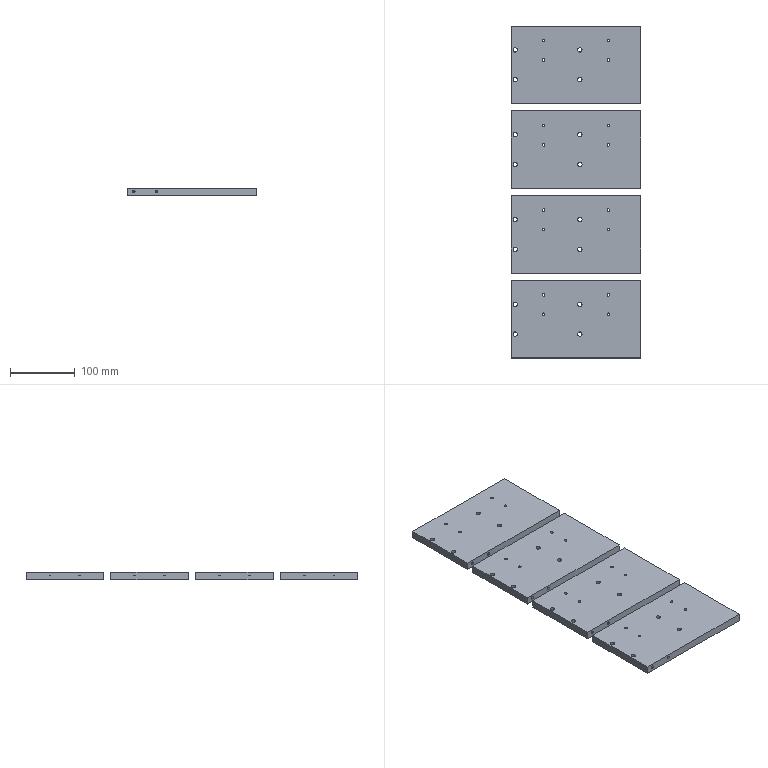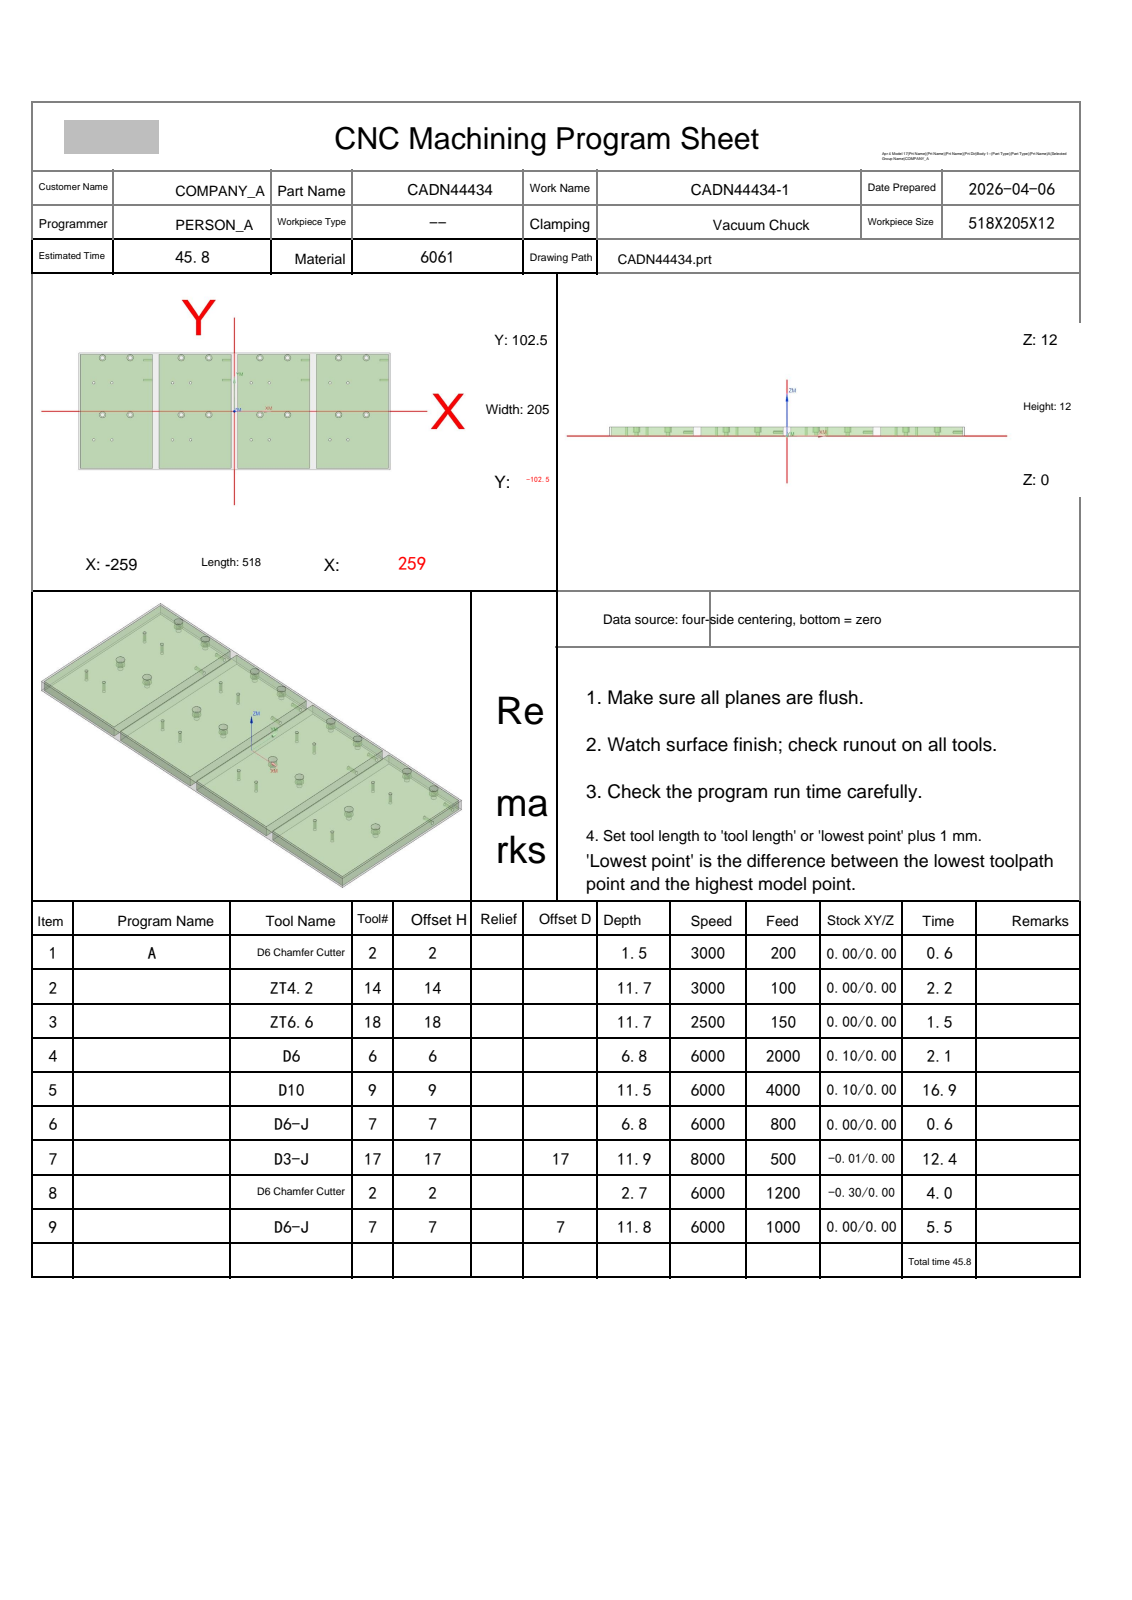NC program | NX | posted by the shop | part box 200 x 513 x 12 mm
Lines 1 to 1643 of 7719, first 1345 of 1641 lines:
%
O0001
(Machine time: 47.09 MIN)
(===Total Tool:7===)
(T2=D6 Chamfer Cutter D=6. R=0. D- H02 Z=9.33  )
(T14=ZT4.2  D=4.2  DR_a=118 D-  H14 Z=0.3   )
(T18=ZT6.6  D=6.6  DR_a=118 D-  H18 Z=0.3   )
(T6=D6      D=6.   R=0.   D-  H06 Z=5.2   )
(T9=D10     D=10.  R=0.   D-  H09 Z=0.5   )
(T7=D6-J    D=6.   R=0.   D-  H07 Z=0.2   )
(T17=D3-J   D=3.   R=0.   D17 H17 Z=0.15  )
G80 G90 G17 G49 G40
G91 G28 Z0
M01
N1 T02 M06
(D6 Chamfer Cutter  D=6. R=0. H=02 ce=0.00 di=0.00)
G00 G90 G54 X-204. Y-50. M03 S3000
G43 H02 Z32.
M08
G98 G81 X-204. Y-50. Z10.5 R13. F200.
X-234.
X-219.5 Y-6.
X-173.5
X-204. Y50.
X-234.
X-219.5 Y94.
X-173.5
X-88.5
X-42.5
X-73. Y50.
X-103.
X-88.5 Y-6.
X-103. Y-50.
X-73.
X-42.5 Y-6.
X28. Y-50.
X58.
X42.5 Y-6.
X88.5
X58. Y50.
X28.
X42.5 Y94.
X88.5
X173.5
X219.5
X189. Y50.
X159.
X173.5 Y-6.
X219.5
X189. Y-50.
X159.
G80
G00 Z32.
G91 G28 Z0.0
M05
M09
G91 G28 Z0.0
M01
N2 T14 M06
(ZT4.2 D=4.2 DR_a=118 H=14)
G00 G90 G54 X-73. Y-50. M03 S3000
G43 H14 Z32.
M08
G98 G83 X-73. Y-50. Z.3 R13. F100. Q1.5
X-103.
X-204.
X-234.
Y50.
X-204.
X-103.
X-73.
X28.
X58.
X159.
X189.
Y-50.
X159.
X58.
X28.
G80
G00 Z32.
G91 G28 Z0.0
M05
M09
G91 G28 Z0.0
M01
N3 T18 M06
(ZT6.6 D=6.6 DR_a=118 H=18)
G00 G90 G54 X219.5 Y94. M03 S2500
G43 H18 Z32.
M08
G98 G83 X219.5 Y94. Z.3 R13. F150. Q3.
X173.5
X88.5
X42.5
X-42.5
X-88.5
X-173.5
X-219.5
Y-6.
X-173.5
X-88.5
X-42.5
X42.5
X88.5
X173.5
X219.5
G80
G00 Z32.
G91 G28 Z0.0
M05
M09
G91 G28 Z0.0
M01
N4 T06 M06
(D6  D=6. R=0. H=06 ce=0.10 di=0.00)
G00 G90 G54 X88.5 Y-6. M03 S6000
G43 H06 Z32.
M08
Z12.3
G03 X87.3 Y-7.2 I0.0 J-1.2 F2000.
X88.5 Y-8.4 I1.2 J0.0
X88.5 Y-8.4 Z11.8 I0.0 J2.4
X88.5 Y-8.4 Z11.3 I0.0 J2.4
X88.5 Y-8.4 Z10.8 I0.0 J2.4
X88.5 Y-8.4 Z10.3 I0.0 J2.4
X88.5 Y-8.4 Z9.8 I0.0 J2.4
X88.5 Y-8.4 Z9.3 I0.0 J2.4
X88.5 Y-8.4 Z8.8 I0.0 J2.4
X88.5 Y-8.4 Z8.3 I0.0 J2.4
X88.5 Y-8.4 Z7.8 I0.0 J2.4
X88.5 Y-8.4 Z7.3 I0.0 J2.4
X88.5 Y-8.4 Z6.8 I0.0 J2.4
X88.5 Y-8.4 Z6.3 I0.0 J2.4
X88.5 Y-8.4 Z5.8 I0.0 J2.4
X88.5 Y-8.4 Z5.3 I0.0 J2.4
X90.783 Y-6.742 Z5.2 I0.0 J2.4
X90.9 Y-6. I-2.283 J.742
X88.5 Y-3.6 I-2.4 J0.0
X86.1 Y-6. I0.0 J-2.4
X88.5 Y-8.4 I2.4 J0.0
X90.783 Y-6.742 I0.0 J2.4
X90.841 Y-6.371 I-1.141 J.371
X89.641 Y-5.171 I-1.2 J0.0
X88.5 Y-6. I0.0 J-1.2
G00 Z32.
X42.5
Z12.3
G03 X41.3 Y-7.2 I0.0 J-1.2
X42.5 Y-8.4 I1.2 J0.0
X42.5 Y-8.4 Z11.8 I0.0 J2.4
X42.5 Y-8.4 Z11.3 I0.0 J2.4
X42.5 Y-8.4 Z10.8 I0.0 J2.4
X42.5 Y-8.4 Z10.3 I0.0 J2.4
X42.5 Y-8.4 Z9.8 I0.0 J2.4
X42.5 Y-8.4 Z9.3 I0.0 J2.4
X42.5 Y-8.4 Z8.8 I0.0 J2.4
X42.5 Y-8.4 Z8.3 I0.0 J2.4
X42.5 Y-8.4 Z7.8 I0.0 J2.4
X42.5 Y-8.4 Z7.3 I0.0 J2.4
X42.5 Y-8.4 Z6.8 I0.0 J2.4
X42.5 Y-8.4 Z6.3 I0.0 J2.4
X42.5 Y-8.4 Z5.8 I0.0 J2.4
X42.5 Y-8.4 Z5.3 I0.0 J2.4
X44.783 Y-6.742 Z5.2 I0.0 J2.4
X44.9 Y-6. I-2.283 J.742
X42.5 Y-3.6 I-2.4 J0.0
X40.1 Y-6. I0.0 J-2.4
X42.5 Y-8.4 I2.4 J0.0
X44.783 Y-6.742 I0.0 J2.4
X44.841 Y-6.371 I-1.141 J.371
X43.641 Y-5.171 I-1.2 J0.0
X42.5 Y-6. I0.0 J-1.2
G00 Z32.
X-42.5
Z12.3
G03 X-43.7 Y-7.2 I0.0 J-1.2
X-42.5 Y-8.4 I1.2 J0.0
X-42.5 Y-8.4 Z11.8 I0.0 J2.4
X-42.5 Y-8.4 Z11.3 I0.0 J2.4
X-42.5 Y-8.4 Z10.8 I0.0 J2.4
X-42.5 Y-8.4 Z10.3 I0.0 J2.4
X-42.5 Y-8.4 Z9.8 I0.0 J2.4
X-42.5 Y-8.4 Z9.3 I0.0 J2.4
X-42.5 Y-8.4 Z8.8 I0.0 J2.4
X-42.5 Y-8.4 Z8.3 I0.0 J2.4
X-42.5 Y-8.4 Z7.8 I0.0 J2.4
X-42.5 Y-8.4 Z7.3 I0.0 J2.4
X-42.5 Y-8.4 Z6.8 I0.0 J2.4
X-42.5 Y-8.4 Z6.3 I0.0 J2.4
X-42.5 Y-8.4 Z5.8 I0.0 J2.4
X-42.5 Y-8.4 Z5.3 I0.0 J2.4
X-40.217 Y-6.742 Z5.2 I0.0 J2.4
X-40.1 Y-6. I-2.283 J.742
X-42.5 Y-3.6 I-2.4 J0.0
X-44.9 Y-6. I0.0 J-2.4
X-42.5 Y-8.4 I2.4 J0.0
X-40.217 Y-6.742 I0.0 J2.4
X-40.159 Y-6.371 I-1.141 J.371
X-41.359 Y-5.171 I-1.2 J0.0
X-42.5 Y-6. I0.0 J-1.2
G00 Z32.
X-88.5
Z12.3
G03 X-89.7 Y-7.2 I0.0 J-1.2
X-88.5 Y-8.4 I1.2 J0.0
X-88.5 Y-8.4 Z11.8 I0.0 J2.4
X-88.5 Y-8.4 Z11.3 I0.0 J2.4
X-88.5 Y-8.4 Z10.8 I0.0 J2.4
X-88.5 Y-8.4 Z10.3 I0.0 J2.4
X-88.5 Y-8.4 Z9.8 I0.0 J2.4
X-88.5 Y-8.4 Z9.3 I0.0 J2.4
X-88.5 Y-8.4 Z8.8 I0.0 J2.4
X-88.5 Y-8.4 Z8.3 I0.0 J2.4
X-88.5 Y-8.4 Z7.8 I0.0 J2.4
X-88.5 Y-8.4 Z7.3 I0.0 J2.4
X-88.5 Y-8.4 Z6.8 I0.0 J2.4
X-88.5 Y-8.4 Z6.3 I0.0 J2.4
X-88.5 Y-8.4 Z5.8 I0.0 J2.4
X-88.5 Y-8.4 Z5.3 I0.0 J2.4
X-86.217 Y-6.742 Z5.2 I0.0 J2.4
X-86.1 Y-6. I-2.283 J.742
X-88.5 Y-3.6 I-2.4 J0.0
X-90.9 Y-6. I0.0 J-2.4
X-88.5 Y-8.4 I2.4 J0.0
X-86.217 Y-6.742 I0.0 J2.4
X-86.159 Y-6.371 I-1.141 J.371
X-87.359 Y-5.171 I-1.2 J0.0
X-88.5 Y-6. I0.0 J-1.2
G00 Z32.
X-173.5
Z12.3
G03 X-174.7 Y-7.2 I0.0 J-1.2
X-173.5 Y-8.4 I1.2 J0.0
X-173.5 Y-8.4 Z11.8 I0.0 J2.4
X-173.5 Y-8.4 Z11.3 I0.0 J2.4
X-173.5 Y-8.4 Z10.8 I0.0 J2.4
X-173.5 Y-8.4 Z10.3 I0.0 J2.4
X-173.5 Y-8.4 Z9.8 I0.0 J2.4
X-173.5 Y-8.4 Z9.3 I0.0 J2.4
X-173.5 Y-8.4 Z8.8 I0.0 J2.4
X-173.5 Y-8.4 Z8.3 I0.0 J2.4
X-173.5 Y-8.4 Z7.8 I0.0 J2.4
X-173.5 Y-8.4 Z7.3 I0.0 J2.4
X-173.5 Y-8.4 Z6.8 I0.0 J2.4
X-173.5 Y-8.4 Z6.3 I0.0 J2.4
X-173.5 Y-8.4 Z5.8 I0.0 J2.4
X-173.5 Y-8.4 Z5.3 I0.0 J2.4
X-171.217 Y-6.742 Z5.2 I0.0 J2.4
X-171.1 Y-6. I-2.283 J.742
X-173.5 Y-3.6 I-2.4 J0.0
X-175.9 Y-6. I0.0 J-2.4
X-173.5 Y-8.4 I2.4 J0.0
X-171.217 Y-6.742 I0.0 J2.4
X-171.159 Y-6.371 I-1.141 J.371
X-172.359 Y-5.171 I-1.2 J0.0
X-173.5 Y-6. I0.0 J-1.2
G00 Z32.
X-219.5
Z12.3
G03 X-220.7 Y-7.2 I0.0 J-1.2
X-219.5 Y-8.4 I1.2 J0.0
X-219.5 Y-8.4 Z11.8 I0.0 J2.4
X-219.5 Y-8.4 Z11.3 I0.0 J2.4
X-219.5 Y-8.4 Z10.8 I0.0 J2.4
X-219.5 Y-8.4 Z10.3 I0.0 J2.4
X-219.5 Y-8.4 Z9.8 I0.0 J2.4
X-219.5 Y-8.4 Z9.3 I0.0 J2.4
X-219.5 Y-8.4 Z8.8 I0.0 J2.4
X-219.5 Y-8.4 Z8.3 I0.0 J2.4
X-219.5 Y-8.4 Z7.8 I0.0 J2.4
X-219.5 Y-8.4 Z7.3 I0.0 J2.4
X-219.5 Y-8.4 Z6.8 I0.0 J2.4
X-219.5 Y-8.4 Z6.3 I0.0 J2.4
X-219.5 Y-8.4 Z5.8 I0.0 J2.4
X-219.5 Y-8.4 Z5.3 I0.0 J2.4
X-217.217 Y-6.742 Z5.2 I0.0 J2.4
X-217.1 Y-6. I-2.283 J.742
X-219.5 Y-3.6 I-2.4 J0.0
X-221.9 Y-6. I0.0 J-2.4
X-219.5 Y-8.4 I2.4 J0.0
X-217.217 Y-6.742 I0.0 J2.4
X-217.159 Y-6.371 I-1.141 J.371
X-218.359 Y-5.171 I-1.2 J0.0
X-219.5 Y-6. I0.0 J-1.2
G00 Z32.
Y94.
Z12.3
G03 X-220.7 Y92.8 I0.0 J-1.2
X-219.5 Y91.6 I1.2 J0.0
X-219.5 Y91.6 Z11.8 I0.0 J2.4
X-219.5 Y91.6 Z11.3 I0.0 J2.4
X-219.5 Y91.6 Z10.8 I0.0 J2.4
X-219.5 Y91.6 Z10.3 I0.0 J2.4
X-219.5 Y91.6 Z9.8 I0.0 J2.4
X-219.5 Y91.6 Z9.3 I0.0 J2.4
X-219.5 Y91.6 Z8.8 I0.0 J2.4
X-219.5 Y91.6 Z8.3 I0.0 J2.4
X-219.5 Y91.6 Z7.8 I0.0 J2.4
X-219.5 Y91.6 Z7.3 I0.0 J2.4
X-219.5 Y91.6 Z6.8 I0.0 J2.4
X-219.5 Y91.6 Z6.3 I0.0 J2.4
X-219.5 Y91.6 Z5.8 I0.0 J2.4
X-219.5 Y91.6 Z5.3 I0.0 J2.4
X-217.217 Y93.258 Z5.2 I0.0 J2.4
X-217.1 Y94. I-2.283 J.742
X-219.5 Y96.4 I-2.4 J0.0
X-221.9 Y94. I0.0 J-2.4
X-219.5 Y91.6 I2.4 J0.0
X-217.217 Y93.258 I0.0 J2.4
X-217.159 Y93.629 I-1.141 J.371
X-218.359 Y94.829 I-1.2 J0.0
X-219.5 Y94. I0.0 J-1.2
G00 Z32.
X-173.5
Z12.3
G03 X-174.7 Y92.8 I0.0 J-1.2
X-173.5 Y91.6 I1.2 J0.0
X-173.5 Y91.6 Z11.8 I0.0 J2.4
X-173.5 Y91.6 Z11.3 I0.0 J2.4
X-173.5 Y91.6 Z10.8 I0.0 J2.4
X-173.5 Y91.6 Z10.3 I0.0 J2.4
X-173.5 Y91.6 Z9.8 I0.0 J2.4
X-173.5 Y91.6 Z9.3 I0.0 J2.4
X-173.5 Y91.6 Z8.8 I0.0 J2.4
X-173.5 Y91.6 Z8.3 I0.0 J2.4
X-173.5 Y91.6 Z7.8 I0.0 J2.4
X-173.5 Y91.6 Z7.3 I0.0 J2.4
X-173.5 Y91.6 Z6.8 I0.0 J2.4
X-173.5 Y91.6 Z6.3 I0.0 J2.4
X-173.5 Y91.6 Z5.8 I0.0 J2.4
X-173.5 Y91.6 Z5.3 I0.0 J2.4
X-171.217 Y93.258 Z5.2 I0.0 J2.4
X-171.1 Y94. I-2.283 J.742
X-173.5 Y96.4 I-2.4 J0.0
X-175.9 Y94. I0.0 J-2.4
X-173.5 Y91.6 I2.4 J0.0
X-171.217 Y93.258 I0.0 J2.4
X-171.159 Y93.629 I-1.141 J.371
X-172.359 Y94.829 I-1.2 J0.0
X-173.5 Y94. I0.0 J-1.2
G00 Z32.
X-88.5
Z12.3
G03 X-89.7 Y92.8 I0.0 J-1.2
X-88.5 Y91.6 I1.2 J0.0
X-88.5 Y91.6 Z11.8 I0.0 J2.4
X-88.5 Y91.6 Z11.3 I0.0 J2.4
X-88.5 Y91.6 Z10.8 I0.0 J2.4
X-88.5 Y91.6 Z10.3 I0.0 J2.4
X-88.5 Y91.6 Z9.8 I0.0 J2.4
X-88.5 Y91.6 Z9.3 I0.0 J2.4
X-88.5 Y91.6 Z8.8 I0.0 J2.4
X-88.5 Y91.6 Z8.3 I0.0 J2.4
X-88.5 Y91.6 Z7.8 I0.0 J2.4
X-88.5 Y91.6 Z7.3 I0.0 J2.4
X-88.5 Y91.6 Z6.8 I0.0 J2.4
X-88.5 Y91.6 Z6.3 I0.0 J2.4
X-88.5 Y91.6 Z5.8 I0.0 J2.4
X-88.5 Y91.6 Z5.3 I0.0 J2.4
X-86.217 Y93.258 Z5.2 I0.0 J2.4
X-86.1 Y94. I-2.283 J.742
X-88.5 Y96.4 I-2.4 J0.0
X-90.9 Y94. I0.0 J-2.4
X-88.5 Y91.6 I2.4 J0.0
X-86.217 Y93.258 I0.0 J2.4
X-86.159 Y93.629 I-1.141 J.371
X-87.359 Y94.829 I-1.2 J0.0
X-88.5 Y94. I0.0 J-1.2
G00 Z32.
X-42.5
Z12.3
G03 X-43.7 Y92.8 I0.0 J-1.2
X-42.5 Y91.6 I1.2 J0.0
X-42.5 Y91.6 Z11.8 I0.0 J2.4
X-42.5 Y91.6 Z11.3 I0.0 J2.4
X-42.5 Y91.6 Z10.8 I0.0 J2.4
X-42.5 Y91.6 Z10.3 I0.0 J2.4
X-42.5 Y91.6 Z9.8 I0.0 J2.4
X-42.5 Y91.6 Z9.3 I0.0 J2.4
X-42.5 Y91.6 Z8.8 I0.0 J2.4
X-42.5 Y91.6 Z8.3 I0.0 J2.4
X-42.5 Y91.6 Z7.8 I0.0 J2.4
X-42.5 Y91.6 Z7.3 I0.0 J2.4
X-42.5 Y91.6 Z6.8 I0.0 J2.4
X-42.5 Y91.6 Z6.3 I0.0 J2.4
X-42.5 Y91.6 Z5.8 I0.0 J2.4
X-42.5 Y91.6 Z5.3 I0.0 J2.4
X-40.217 Y93.258 Z5.2 I0.0 J2.4
X-40.1 Y94. I-2.283 J.742
X-42.5 Y96.4 I-2.4 J0.0
X-44.9 Y94. I0.0 J-2.4
X-42.5 Y91.6 I2.4 J0.0
X-40.217 Y93.258 I0.0 J2.4
X-40.159 Y93.629 I-1.141 J.371
X-41.359 Y94.829 I-1.2 J0.0
X-42.5 Y94. I0.0 J-1.2
G00 Z32.
X42.5
Z12.3
G03 X41.3 Y92.8 I0.0 J-1.2
X42.5 Y91.6 I1.2 J0.0
X42.5 Y91.6 Z11.8 I0.0 J2.4
X42.5 Y91.6 Z11.3 I0.0 J2.4
X42.5 Y91.6 Z10.8 I0.0 J2.4
X42.5 Y91.6 Z10.3 I0.0 J2.4
X42.5 Y91.6 Z9.8 I0.0 J2.4
X42.5 Y91.6 Z9.3 I0.0 J2.4
X42.5 Y91.6 Z8.8 I0.0 J2.4
X42.5 Y91.6 Z8.3 I0.0 J2.4
X42.5 Y91.6 Z7.8 I0.0 J2.4
X42.5 Y91.6 Z7.3 I0.0 J2.4
X42.5 Y91.6 Z6.8 I0.0 J2.4
X42.5 Y91.6 Z6.3 I0.0 J2.4
X42.5 Y91.6 Z5.8 I0.0 J2.4
X42.5 Y91.6 Z5.3 I0.0 J2.4
X44.783 Y93.258 Z5.2 I0.0 J2.4
X44.9 Y94. I-2.283 J.742
X42.5 Y96.4 I-2.4 J0.0
X40.1 Y94. I0.0 J-2.4
X42.5 Y91.6 I2.4 J0.0
X44.783 Y93.258 I0.0 J2.4
X44.841 Y93.629 I-1.141 J.371
X43.641 Y94.829 I-1.2 J0.0
X42.5 Y94. I0.0 J-1.2
G00 Z32.
X88.5
Z12.3
G03 X87.3 Y92.8 I0.0 J-1.2
X88.5 Y91.6 I1.2 J0.0
X88.5 Y91.6 Z11.8 I0.0 J2.4
X88.5 Y91.6 Z11.3 I0.0 J2.4
X88.5 Y91.6 Z10.8 I0.0 J2.4
X88.5 Y91.6 Z10.3 I0.0 J2.4
X88.5 Y91.6 Z9.8 I0.0 J2.4
X88.5 Y91.6 Z9.3 I0.0 J2.4
X88.5 Y91.6 Z8.8 I0.0 J2.4
X88.5 Y91.6 Z8.3 I0.0 J2.4
X88.5 Y91.6 Z7.8 I0.0 J2.4
X88.5 Y91.6 Z7.3 I0.0 J2.4
X88.5 Y91.6 Z6.8 I0.0 J2.4
X88.5 Y91.6 Z6.3 I0.0 J2.4
X88.5 Y91.6 Z5.8 I0.0 J2.4
X88.5 Y91.6 Z5.3 I0.0 J2.4
X90.783 Y93.258 Z5.2 I0.0 J2.4
X90.9 Y94. I-2.283 J.742
X88.5 Y96.4 I-2.4 J0.0
X86.1 Y94. I0.0 J-2.4
X88.5 Y91.6 I2.4 J0.0
X90.783 Y93.258 I0.0 J2.4
X90.841 Y93.629 I-1.141 J.371
X89.641 Y94.829 I-1.2 J0.0
X88.5 Y94. I0.0 J-1.2
G00 Z32.
X173.5
Z12.3
G03 X172.3 Y92.8 I0.0 J-1.2
X173.5 Y91.6 I1.2 J0.0
X173.5 Y91.6 Z11.8 I0.0 J2.4
X173.5 Y91.6 Z11.3 I0.0 J2.4
X173.5 Y91.6 Z10.8 I0.0 J2.4
X173.5 Y91.6 Z10.3 I0.0 J2.4
X173.5 Y91.6 Z9.8 I0.0 J2.4
X173.5 Y91.6 Z9.3 I0.0 J2.4
X173.5 Y91.6 Z8.8 I0.0 J2.4
X173.5 Y91.6 Z8.3 I0.0 J2.4
X173.5 Y91.6 Z7.8 I0.0 J2.4
X173.5 Y91.6 Z7.3 I0.0 J2.4
X173.5 Y91.6 Z6.8 I0.0 J2.4
X173.5 Y91.6 Z6.3 I0.0 J2.4
X173.5 Y91.6 Z5.8 I0.0 J2.4
X173.5 Y91.6 Z5.3 I0.0 J2.4
X175.783 Y93.258 Z5.2 I0.0 J2.4
X175.9 Y94. I-2.283 J.742
X173.5 Y96.4 I-2.4 J0.0
X171.1 Y94. I0.0 J-2.4
X173.5 Y91.6 I2.4 J0.0
X175.783 Y93.258 I0.0 J2.4
X175.841 Y93.629 I-1.141 J.371
X174.641 Y94.829 I-1.2 J0.0
X173.5 Y94. I0.0 J-1.2
G00 Z32.
X219.5
Z12.3
G03 X218.3 Y92.8 I0.0 J-1.2
X219.5 Y91.6 I1.2 J0.0
X219.5 Y91.6 Z11.8 I0.0 J2.4
X219.5 Y91.6 Z11.3 I0.0 J2.4
X219.5 Y91.6 Z10.8 I0.0 J2.4
X219.5 Y91.6 Z10.3 I0.0 J2.4
X219.5 Y91.6 Z9.8 I0.0 J2.4
X219.5 Y91.6 Z9.3 I0.0 J2.4
X219.5 Y91.6 Z8.8 I0.0 J2.4
X219.5 Y91.6 Z8.3 I0.0 J2.4
X219.5 Y91.6 Z7.8 I0.0 J2.4
X219.5 Y91.6 Z7.3 I0.0 J2.4
X219.5 Y91.6 Z6.8 I0.0 J2.4
X219.5 Y91.6 Z6.3 I0.0 J2.4
X219.5 Y91.6 Z5.8 I0.0 J2.4
X219.5 Y91.6 Z5.3 I0.0 J2.4
X221.783 Y93.258 Z5.2 I0.0 J2.4
X221.9 Y94. I-2.283 J.742
X219.5 Y96.4 I-2.4 J0.0
X217.1 Y94. I0.0 J-2.4
X219.5 Y91.6 I2.4 J0.0
X221.783 Y93.258 I0.0 J2.4
X221.841 Y93.629 I-1.141 J.371
X220.641 Y94.829 I-1.2 J0.0
X219.5 Y94. I0.0 J-1.2
G00 Z32.
Y-6.
Z12.3
G03 X218.3 Y-7.2 I0.0 J-1.2
X219.5 Y-8.4 I1.2 J0.0
X219.5 Y-8.4 Z11.8 I0.0 J2.4
X219.5 Y-8.4 Z11.3 I0.0 J2.4
X219.5 Y-8.4 Z10.8 I0.0 J2.4
X219.5 Y-8.4 Z10.3 I0.0 J2.4
X219.5 Y-8.4 Z9.8 I0.0 J2.4
X219.5 Y-8.4 Z9.3 I0.0 J2.4
X219.5 Y-8.4 Z8.8 I0.0 J2.4
X219.5 Y-8.4 Z8.3 I0.0 J2.4
X219.5 Y-8.4 Z7.8 I0.0 J2.4
X219.5 Y-8.4 Z7.3 I0.0 J2.4
X219.5 Y-8.4 Z6.8 I0.0 J2.4
X219.5 Y-8.4 Z6.3 I0.0 J2.4
X219.5 Y-8.4 Z5.8 I0.0 J2.4
X219.5 Y-8.4 Z5.3 I0.0 J2.4
X221.783 Y-6.742 Z5.2 I0.0 J2.4
X221.9 Y-6. I-2.283 J.742
X219.5 Y-3.6 I-2.4 J0.0
X217.1 Y-6. I0.0 J-2.4
X219.5 Y-8.4 I2.4 J0.0
X221.783 Y-6.742 I0.0 J2.4
X221.841 Y-6.371 I-1.141 J.371
X220.641 Y-5.171 I-1.2 J0.0
X219.5 Y-6. I0.0 J-1.2
G00 Z32.
X173.5
Z12.3
G03 X172.3 Y-7.2 I0.0 J-1.2
X173.5 Y-8.4 I1.2 J0.0
X173.5 Y-8.4 Z11.8 I0.0 J2.4
X173.5 Y-8.4 Z11.3 I0.0 J2.4
X173.5 Y-8.4 Z10.8 I0.0 J2.4
X173.5 Y-8.4 Z10.3 I0.0 J2.4
X173.5 Y-8.4 Z9.8 I0.0 J2.4
X173.5 Y-8.4 Z9.3 I0.0 J2.4
X173.5 Y-8.4 Z8.8 I0.0 J2.4
X173.5 Y-8.4 Z8.3 I0.0 J2.4
X173.5 Y-8.4 Z7.8 I0.0 J2.4
X173.5 Y-8.4 Z7.3 I0.0 J2.4
X173.5 Y-8.4 Z6.8 I0.0 J2.4
X173.5 Y-8.4 Z6.3 I0.0 J2.4
X173.5 Y-8.4 Z5.8 I0.0 J2.4
X173.5 Y-8.4 Z5.3 I0.0 J2.4
X175.783 Y-6.742 Z5.2 I0.0 J2.4
X175.9 Y-6. I-2.283 J.742
X173.5 Y-3.6 I-2.4 J0.0
X171.1 Y-6. I0.0 J-2.4
X173.5 Y-8.4 I2.4 J0.0
X175.783 Y-6.742 I0.0 J2.4
X175.841 Y-6.371 I-1.141 J.371
X174.641 Y-5.171 I-1.2 J0.0
X173.5 Y-6. I0.0 J-1.2
G00 Z32.
G91 G28 Z0.0
M05
M09
G91 G28 Z0.0
M01
N5 T09 M06
(D10  D=10. R=0. H=09 ce=0.10 di=0.00)
G00 G90 G54 X-130.6 Y0.0 M03 S6000
G43 H09 Z32.
M08
Z12.5
G01 Y100. Z12.426 F4000.
G02 X-125.5 Y105.1 Z12.42 I5.1 J0.0
G01 X-5.5 Z12.33
G02 X-.4 Y100. Z12.324 I0.0 J-5.1
G01 Y-100. Z12.176
G02 X-5.5 Y-105.1 Z12.17 I-5.1 J0.0
G01 X-125.5 Z12.08
G02 X-130.6 Y-100. Z12.074 I0.0 J5.1
G01 Y100. Z11.926
G02 X-125.5 Y105.1 Z11.92 I5.1 J0.0
G01 X-5.5 Z11.83
G02 X-.4 Y100. Z11.824 I0.0 J-5.1
G01 Y-100. Z11.676
G02 X-5.5 Y-105.1 Z11.67 I-5.1 J0.0
G01 X-125.5 Z11.58
G02 X-130.6 Y-100. Z11.574 I0.0 J5.1
G01 Y100. Z11.426
G02 X-125.5 Y105.1 Z11.42 I5.1 J0.0
G01 X-5.5 Z11.33
G02 X-.4 Y100. Z11.324 I0.0 J-5.1
G01 Y-100. Z11.176
G02 X-5.5 Y-105.1 Z11.17 I-5.1 J0.0
G01 X-125.5 Z11.08
G02 X-130.6 Y-100. Z11.074 I0.0 J5.1
G01 Y100. Z10.926
G02 X-125.5 Y105.1 Z10.92 I5.1 J0.0
G01 X-5.5 Z10.83
G02 X-.4 Y100. Z10.824 I0.0 J-5.1
G01 Y-100. Z10.676
G02 X-5.5 Y-105.1 Z10.67 I-5.1 J0.0
G01 X-125.5 Z10.58
G02 X-130.6 Y-100. Z10.574 I0.0 J5.1
G01 Y100. Z10.426
G02 X-125.5 Y105.1 Z10.42 I5.1 J0.0
G01 X-5.5 Z10.33
G02 X-.4 Y100. Z10.324 I0.0 J-5.1
G01 Y-100. Z10.176
G02 X-5.5 Y-105.1 Z10.17 I-5.1 J0.0
G01 X-125.5 Z10.08
G02 X-130.6 Y-100. Z10.074 I0.0 J5.1
G01 Y100. Z9.926
G02 X-125.5 Y105.1 Z9.92 I5.1 J0.0
G01 X-5.5 Z9.83
G02 X-.4 Y100. Z9.824 I0.0 J-5.1
G01 Y-100. Z9.676
G02 X-5.5 Y-105.1 Z9.67 I-5.1 J0.0
G01 X-125.5 Z9.58
G02 X-130.6 Y-100. Z9.574 I0.0 J5.1
G01 Y100. Z9.426
G02 X-125.5 Y105.1 Z9.42 I5.1 J0.0
G01 X-5.5 Z9.33
G02 X-.4 Y100. Z9.324 I0.0 J-5.1
G01 Y-100. Z9.176
G02 X-5.5 Y-105.1 Z9.17 I-5.1 J0.0
G01 X-125.5 Z9.08
G02 X-130.6 Y-100. Z9.074 I0.0 J5.1
G01 Y100. Z8.926
G02 X-125.5 Y105.1 Z8.92 I5.1 J0.0
G01 X-5.5 Z8.83
G02 X-.4 Y100. Z8.824 I0.0 J-5.1
G01 Y-100. Z8.676
G02 X-5.5 Y-105.1 Z8.67 I-5.1 J0.0
G01 X-125.5 Z8.58
G02 X-130.6 Y-100. Z8.574 I0.0 J5.1
G01 Y100. Z8.426
G02 X-125.5 Y105.1 Z8.42 I5.1 J0.0
G01 X-5.5 Z8.33
G02 X-.4 Y100. Z8.324 I0.0 J-5.1
G01 Y-100. Z8.176
G02 X-5.5 Y-105.1 Z8.17 I-5.1 J0.0
G01 X-125.5 Z8.08
G02 X-130.6 Y-100. Z8.074 I0.0 J5.1
G01 Y100. Z7.926
G02 X-125.5 Y105.1 Z7.92 I5.1 J0.0
G01 X-5.5 Z7.83
G02 X-.4 Y100. Z7.824 I0.0 J-5.1
G01 Y-100. Z7.676
G02 X-5.5 Y-105.1 Z7.67 I-5.1 J0.0
G01 X-125.5 Z7.58
G02 X-130.6 Y-100. Z7.574 I0.0 J5.1
G01 Y100. Z7.426
G02 X-125.5 Y105.1 Z7.42 I5.1 J0.0
G01 X-5.5 Z7.33
G02 X-.4 Y100. Z7.324 I0.0 J-5.1
G01 Y-100. Z7.176
G02 X-5.5 Y-105.1 Z7.17 I-5.1 J0.0
G01 X-125.5 Z7.08
G02 X-130.6 Y-100. Z7.074 I0.0 J5.1
G01 Y100. Z6.926
G02 X-125.5 Y105.1 Z6.92 I5.1 J0.0
G01 X-5.5 Z6.83
G02 X-.4 Y100. Z6.824 I0.0 J-5.1
G01 Y-100. Z6.676
G02 X-5.5 Y-105.1 Z6.67 I-5.1 J0.0
G01 X-125.5 Z6.58
G02 X-130.6 Y-100. Z6.574 I0.0 J5.1
G01 Y100. Z6.426
G02 X-125.5 Y105.1 Z6.42 I5.1 J0.0
G01 X-5.5 Z6.33
G02 X-.4 Y100. Z6.324 I0.0 J-5.1
G01 Y-100. Z6.176
G02 X-5.5 Y-105.1 Z6.17 I-5.1 J0.0
G01 X-125.5 Z6.08
G02 X-130.6 Y-100. Z6.074 I0.0 J5.1
G01 Y100. Z5.926
G02 X-125.5 Y105.1 Z5.92 I5.1 J0.0
G01 X-5.5 Z5.83
G02 X-.4 Y100. Z5.824 I0.0 J-5.1
G01 Y-100. Z5.676
G02 X-5.5 Y-105.1 Z5.67 I-5.1 J0.0
G01 X-125.5 Z5.58
G02 X-130.6 Y-100. Z5.574 I0.0 J5.1
G01 Y100. Z5.426
G02 X-125.5 Y105.1 Z5.42 I5.1 J0.0
G01 X-5.5 Z5.33
G02 X-.4 Y100. Z5.324 I0.0 J-5.1
G01 Y-100. Z5.176
G02 X-5.5 Y-105.1 Z5.17 I-5.1 J0.0
G01 X-125.5 Z5.08
G02 X-130.6 Y-100. Z5.074 I0.0 J5.1
G01 Y100. Z4.926
G02 X-125.5 Y105.1 Z4.92 I5.1 J0.0
G01 X-5.5 Z4.83
G02 X-.4 Y100. Z4.824 I0.0 J-5.1
G01 Y-100. Z4.676
G02 X-5.5 Y-105.1 Z4.67 I-5.1 J0.0
G01 X-125.5 Z4.58
G02 X-130.6 Y-100. Z4.574 I0.0 J5.1
G01 Y100. Z4.426
G02 X-125.5 Y105.1 Z4.42 I5.1 J0.0
G01 X-5.5 Z4.33
G02 X-.4 Y100. Z4.324 I0.0 J-5.1
G01 Y-100. Z4.176
G02 X-5.5 Y-105.1 Z4.17 I-5.1 J0.0
G01 X-125.5 Z4.08
G02 X-130.6 Y-100. Z4.074 I0.0 J5.1
G01 Y100. Z3.926
G02 X-125.5 Y105.1 Z3.92 I5.1 J0.0
G01 X-5.5 Z3.83
G02 X-.4 Y100. Z3.824 I0.0 J-5.1
G01 Y-100. Z3.676
G02 X-5.5 Y-105.1 Z3.67 I-5.1 J0.0
G01 X-125.5 Z3.58
G02 X-130.6 Y-100. Z3.574 I0.0 J5.1
G01 Y100. Z3.426
G02 X-125.5 Y105.1 Z3.42 I5.1 J0.0
G01 X-5.5 Z3.33
G02 X-.4 Y100. Z3.324 I0.0 J-5.1
G01 Y-100. Z3.176
G02 X-5.5 Y-105.1 Z3.17 I-5.1 J0.0
G01 X-125.5 Z3.08
G02 X-130.6 Y-100. Z3.074 I0.0 J5.1
G01 Y100. Z2.926
G02 X-125.5 Y105.1 Z2.92 I5.1 J0.0
G01 X-5.5 Z2.83
G02 X-.4 Y100. Z2.824 I0.0 J-5.1
G01 Y-100. Z2.676
G02 X-5.5 Y-105.1 Z2.67 I-5.1 J0.0
G01 X-125.5 Z2.58
G02 X-130.6 Y-100. Z2.574 I0.0 J5.1
G01 Y100. Z2.426
G02 X-125.5 Y105.1 Z2.42 I5.1 J0.0
G01 X-5.5 Z2.33
G02 X-.4 Y100. Z2.324 I0.0 J-5.1
G01 Y-100. Z2.176
G02 X-5.5 Y-105.1 Z2.17 I-5.1 J0.0
G01 X-125.5 Z2.08
G02 X-130.6 Y-100. Z2.074 I0.0 J5.1
G01 Y100. Z1.926
G02 X-125.5 Y105.1 Z1.92 I5.1 J0.0
G01 X-5.5 Z1.83
G02 X-.4 Y100. Z1.824 I0.0 J-5.1
G01 Y-100. Z1.676
G02 X-5.5 Y-105.1 Z1.67 I-5.1 J0.0
G01 X-125.5 Z1.58
G02 X-130.6 Y-100. Z1.574 I0.0 J5.1
G01 Y100. Z1.426
G02 X-125.5 Y105.1 Z1.42 I5.1 J0.0
G01 X-5.5 Z1.33
G02 X-.4 Y100. Z1.324 I0.0 J-5.1
G01 Y-100. Z1.176
G02 X-5.5 Y-105.1 Z1.17 I-5.1 J0.0
G01 X-125.5 Z1.08
G02 X-130.6 Y-100. Z1.074 I0.0 J5.1
G01 Y100. Z.926
G02 X-125.5 Y105.1 Z.92 I5.1 J0.0
G01 X-5.5 Z.83
G02 X-.4 Y100. Z.824 I0.0 J-5.1
G01 Y-100. Z.676
G02 X-5.5 Y-105.1 Z.67 I-5.1 J0.0
G01 X-125.5 Z.58
G02 X-130.6 Y-100. Z.574 I0.0 J5.1
G01 Y0.0 Z.5
Y100.
G02 X-125.5 Y105.1 I5.1 J0.0
G01 X-5.5
G02 X-.4 Y100. I0.0 J-5.1
G01 Y-100.
G02 X-5.5 Y-105.1 I-5.1 J0.0
G01 X-125.5
G02 X-130.6 Y-100. I0.0 J5.1
G01 Y0.0
Y.5
Z1.5
G00 Z32.
X-261.6 Y0.0
Z12.5
G01 Y100. Z12.426
G02 X-256.5 Y105.1 Z12.42 I5.1 J0.0
G01 X-136.5 Z12.33
G02 X-131.4 Y100. Z12.324 I0.0 J-5.1
G01 Y-100. Z12.176
G02 X-136.5 Y-105.1 Z12.17 I-5.1 J0.0
G01 X-256.5 Z12.08
G02 X-261.6 Y-100. Z12.074 I0.0 J5.1
G01 Y100. Z11.926
G02 X-256.5 Y105.1 Z11.92 I5.1 J0.0
G01 X-136.5 Z11.83
G02 X-131.4 Y100. Z11.824 I0.0 J-5.1
G01 Y-100. Z11.676
G02 X-136.5 Y-105.1 Z11.67 I-5.1 J0.0
G01 X-256.5 Z11.58
G02 X-261.6 Y-100. Z11.574 I0.0 J5.1
G01 Y100. Z11.426
G02 X-256.5 Y105.1 Z11.42 I5.1 J0.0
G01 X-136.5 Z11.33
G02 X-131.4 Y100. Z11.324 I0.0 J-5.1
G01 Y-100. Z11.176
G02 X-136.5 Y-105.1 Z11.17 I-5.1 J0.0
G01 X-256.5 Z11.08
G02 X-261.6 Y-100. Z11.074 I0.0 J5.1
G01 Y100. Z10.926
G02 X-256.5 Y105.1 Z10.92 I5.1 J0.0
G01 X-136.5 Z10.83
G02 X-131.4 Y100. Z10.824 I0.0 J-5.1
G01 Y-100. Z10.676
G02 X-136.5 Y-105.1 Z10.67 I-5.1 J0.0
G01 X-256.5 Z10.58
G02 X-261.6 Y-100. Z10.574 I0.0 J5.1
G01 Y100. Z10.426
G02 X-256.5 Y105.1 Z10.42 I5.1 J0.0
G01 X-136.5 Z10.33
G02 X-131.4 Y100. Z10.324 I0.0 J-5.1
G01 Y-100. Z10.176
G02 X-136.5 Y-105.1 Z10.17 I-5.1 J0.0
G01 X-256.5 Z10.08
G02 X-261.6 Y-100. Z10.074 I0.0 J5.1
G01 Y100. Z9.926
G02 X-256.5 Y105.1 Z9.92 I5.1 J0.0
G01 X-136.5 Z9.83
G02 X-131.4 Y100. Z9.824 I0.0 J-5.1
G01 Y-100. Z9.676
G02 X-136.5 Y-105.1 Z9.67 I-5.1 J0.0
G01 X-256.5 Z9.58
G02 X-261.6 Y-100. Z9.574 I0.0 J5.1
G01 Y100. Z9.426
G02 X-256.5 Y105.1 Z9.42 I5.1 J0.0
G01 X-136.5 Z9.33
G02 X-131.4 Y100. Z9.324 I0.0 J-5.1
G01 Y-100. Z9.176
G02 X-136.5 Y-105.1 Z9.17 I-5.1 J0.0
G01 X-256.5 Z9.08
G02 X-261.6 Y-100. Z9.074 I0.0 J5.1
G01 Y100. Z8.926
G02 X-256.5 Y105.1 Z8.92 I5.1 J0.0
G01 X-136.5 Z8.83
G02 X-131.4 Y100. Z8.824 I0.0 J-5.1
G01 Y-100. Z8.676
G02 X-136.5 Y-105.1 Z8.67 I-5.1 J0.0
G01 X-256.5 Z8.58
G02 X-261.6 Y-100. Z8.574 I0.0 J5.1
G01 Y100. Z8.426
G02 X-256.5 Y105.1 Z8.42 I5.1 J0.0
G01 X-136.5 Z8.33
G02 X-131.4 Y100. Z8.324 I0.0 J-5.1
G01 Y-100. Z8.176
G02 X-136.5 Y-105.1 Z8.17 I-5.1 J0.0
G01 X-256.5 Z8.08
G02 X-261.6 Y-100. Z8.074 I0.0 J5.1
G01 Y100. Z7.926
G02 X-256.5 Y105.1 Z7.92 I5.1 J0.0
G01 X-136.5 Z7.83
G02 X-131.4 Y100. Z7.824 I0.0 J-5.1
G01 Y-100. Z7.676
G02 X-136.5 Y-105.1 Z7.67 I-5.1 J0.0
G01 X-256.5 Z7.58
G02 X-261.6 Y-100. Z7.574 I0.0 J5.1
G01 Y100. Z7.426
G02 X-256.5 Y105.1 Z7.42 I5.1 J0.0
G01 X-136.5 Z7.33
G02 X-131.4 Y100. Z7.324 I0.0 J-5.1
G01 Y-100. Z7.176
G02 X-136.5 Y-105.1 Z7.17 I-5.1 J0.0
G01 X-256.5 Z7.08
G02 X-261.6 Y-100. Z7.074 I0.0 J5.1
G01 Y100. Z6.926
G02 X-256.5 Y105.1 Z6.92 I5.1 J0.0
G01 X-136.5 Z6.83
G02 X-131.4 Y100. Z6.824 I0.0 J-5.1
G01 Y-100. Z6.676
G02 X-136.5 Y-105.1 Z6.67 I-5.1 J0.0
G01 X-256.5 Z6.58
G02 X-261.6 Y-100. Z6.574 I0.0 J5.1
G01 Y100. Z6.426
G02 X-256.5 Y105.1 Z6.42 I5.1 J0.0
G01 X-136.5 Z6.33
G02 X-131.4 Y100. Z6.324 I0.0 J-5.1
G01 Y-100. Z6.176
G02 X-136.5 Y-105.1 Z6.17 I-5.1 J0.0
G01 X-256.5 Z6.08
G02 X-261.6 Y-100. Z6.074 I0.0 J5.1
G01 Y100. Z5.926
G02 X-256.5 Y105.1 Z5.92 I5.1 J0.0
G01 X-136.5 Z5.83
G02 X-131.4 Y100. Z5.824 I0.0 J-5.1
G01 Y-100. Z5.676
G02 X-136.5 Y-105.1 Z5.67 I-5.1 J0.0
G01 X-256.5 Z5.58
G02 X-261.6 Y-100. Z5.574 I0.0 J5.1
G01 Y100. Z5.426
G02 X-256.5 Y105.1 Z5.42 I5.1 J0.0
G01 X-136.5 Z5.33
G02 X-131.4 Y100. Z5.324 I0.0 J-5.1
G01 Y-100. Z5.176
G02 X-136.5 Y-105.1 Z5.17 I-5.1 J0.0
G01 X-256.5 Z5.08
G02 X-261.6 Y-100. Z5.074 I0.0 J5.1
G01 Y100. Z4.926
G02 X-256.5 Y105.1 Z4.92 I5.1 J0.0
G01 X-136.5 Z4.83
G02 X-131.4 Y100. Z4.824 I0.0 J-5.1
G01 Y-100. Z4.676
G02 X-136.5 Y-105.1 Z4.67 I-5.1 J0.0
G01 X-256.5 Z4.58
G02 X-261.6 Y-100. Z4.574 I0.0 J5.1
G01 Y100. Z4.426
G02 X-256.5 Y105.1 Z4.42 I5.1 J0.0
G01 X-136.5 Z4.33
G02 X-131.4 Y100. Z4.324 I0.0 J-5.1
G01 Y-100. Z4.176
G02 X-136.5 Y-105.1 Z4.17 I-5.1 J0.0
G01 X-256.5 Z4.08
G02 X-261.6 Y-100. Z4.074 I0.0 J5.1
G01 Y100. Z3.926
G02 X-256.5 Y105.1 Z3.92 I5.1 J0.0
G01 X-136.5 Z3.83
G02 X-131.4 Y100. Z3.824 I0.0 J-5.1
G01 Y-100. Z3.676
G02 X-136.5 Y-105.1 Z3.67 I-5.1 J0.0
G01 X-256.5 Z3.58
G02 X-261.6 Y-100. Z3.574 I0.0 J5.1
G01 Y100. Z3.426
G02 X-256.5 Y105.1 Z3.42 I5.1 J0.0
G01 X-136.5 Z3.33
G02 X-131.4 Y100. Z3.324 I0.0 J-5.1
G01 Y-100. Z3.176
G02 X-136.5 Y-105.1 Z3.17 I-5.1 J0.0
G01 X-256.5 Z3.08
G02 X-261.6 Y-100. Z3.074 I0.0 J5.1
G01 Y100. Z2.926
G02 X-256.5 Y105.1 Z2.92 I5.1 J0.0
G01 X-136.5 Z2.83
G02 X-131.4 Y100. Z2.824 I0.0 J-5.1
G01 Y-100. Z2.676
G02 X-136.5 Y-105.1 Z2.67 I-5.1 J0.0
G01 X-256.5 Z2.58
G02 X-261.6 Y-100. Z2.574 I0.0 J5.1
G01 Y100. Z2.426
G02 X-256.5 Y105.1 Z2.42 I5.1 J0.0
G01 X-136.5 Z2.33
G02 X-131.4 Y100. Z2.324 I0.0 J-5.1
G01 Y-100. Z2.176
G02 X-136.5 Y-105.1 Z2.17 I-5.1 J0.0
G01 X-256.5 Z2.08
G02 X-261.6 Y-100. Z2.074 I0.0 J5.1
G01 Y100. Z1.926
G02 X-256.5 Y105.1 Z1.92 I5.1 J0.0
G01 X-136.5 Z1.83
G02 X-131.4 Y100. Z1.824 I0.0 J-5.1
G01 Y-100. Z1.676
G02 X-136.5 Y-105.1 Z1.67 I-5.1 J0.0
G01 X-256.5 Z1.58
G02 X-261.6 Y-100. Z1.574 I0.0 J5.1
G01 Y100. Z1.426
G02 X-256.5 Y105.1 Z1.42 I5.1 J0.0
G01 X-136.5 Z1.33
G02 X-131.4 Y100. Z1.324 I0.0 J-5.1
G01 Y-100. Z1.176
G02 X-136.5 Y-105.1 Z1.17 I-5.1 J0.0
G01 X-256.5 Z1.08
G02 X-261.6 Y-100. Z1.074 I0.0 J5.1
G01 Y100. Z.926
G02 X-256.5 Y105.1 Z.92 I5.1 J0.0
G01 X-136.5 Z.83
G02 X-131.4 Y100. Z.824 I0.0 J-5.1
G01 Y-100. Z.676
G02 X-136.5 Y-105.1 Z.67 I-5.1 J0.0
G01 X-256.5 Z.58
G02 X-261.6 Y-100. Z.574 I0.0 J5.1
G01 Y0.0 Z.5
Y100.
G02 X-256.5 Y105.1 I5.1 J0.0
G01 X-136.5
G02 X-131.4 Y100. I0.0 J-5.1
G01 Y-100.
G02 X-136.5 Y-105.1 I-5.1 J0.0
G01 X-256.5
G02 X-261.6 Y-100. I0.0 J5.1
G01 Y0.0
Y.5
Z1.5
G00 Z32.
X.4 Y0.0
Z12.5
G01 Y100. Z12.426
G02 X5.5 Y105.1 Z12.42 I5.1 J0.0
G01 X125.5 Z12.33
G02 X130.6 Y100. Z12.324 I0.0 J-5.1
G01 Y-100. Z12.176
G02 X125.5 Y-105.1 Z12.17 I-5.1 J0.0
G01 X5.5 Z12.08
G02 X.4 Y-100. Z12.074 I0.0 J5.1
G01 Y100. Z11.926
G02 X5.5 Y105.1 Z11.92 I5.1 J0.0
G01 X125.5 Z11.83
G02 X130.6 Y100. Z11.824 I0.0 J-5.1
G01 Y-100. Z11.676
G02 X125.5 Y-105.1 Z11.67 I-5.1 J0.0
G01 X5.5 Z11.58
G02 X.4 Y-100. Z11.574 I0.0 J5.1
G01 Y100. Z11.426
G02 X5.5 Y105.1 Z11.42 I5.1 J0.0
G01 X125.5 Z11.33
G02 X130.6 Y100. Z11.324 I0.0 J-5.1
G01 Y-100. Z11.176
G02 X125.5 Y-105.1 Z11.17 I-5.1 J0.0
G01 X5.5 Z11.08
G02 X.4 Y-100. Z11.074 I0.0 J5.1
G01 Y100. Z10.926
G02 X5.5 Y105.1 Z10.92 I5.1 J0.0
G01 X125.5 Z10.83
G02 X130.6 Y100. Z10.824 I0.0 J-5.1
G01 Y-100. Z10.676
G02 X125.5 Y-105.1 Z10.67 I-5.1 J0.0
G01 X5.5 Z10.58
G02 X.4 Y-100. Z10.574 I0.0 J5.1
G01 Y100. Z10.426
G02 X5.5 Y105.1 Z10.42 I5.1 J0.0
G01 X125.5 Z10.33
G02 X130.6 Y100. Z10.324 I0.0 J-5.1
G01 Y-100. Z10.176
G02 X125.5 Y-105.1 Z10.17 I-5.1 J0.0
G01 X5.5 Z10.08
G02 X.4 Y-100. Z10.074 I0.0 J5.1
G01 Y100. Z9.926
G02 X5.5 Y105.1 Z9.92 I5.1 J0.0
G01 X125.5 Z9.83
G02 X130.6 Y100. Z9.824 I0.0 J-5.1
G01 Y-100. Z9.676
G02 X125.5 Y-105.1 Z9.67 I-5.1 J0.0
G01 X5.5 Z9.58
G02 X.4 Y-100. Z9.574 I0.0 J5.1
G01 Y100. Z9.426
G02 X5.5 Y105.1 Z9.42 I5.1 J0.0
G01 X125.5 Z9.33
G02 X130.6 Y100. Z9.324 I0.0 J-5.1
G01 Y-100. Z9.176
G02 X125.5 Y-105.1 Z9.17 I-5.1 J0.0
G01 X5.5 Z9.08
G02 X.4 Y-100. Z9.074 I0.0 J5.1
G01 Y100. Z8.926
G02 X5.5 Y105.1 Z8.92 I5.1 J0.0
G01 X125.5 Z8.83
G02 X130.6 Y100. Z8.824 I0.0 J-5.1
G01 Y-100. Z8.676
G02 X125.5 Y-105.1 Z8.67 I-5.1 J0.0
G01 X5.5 Z8.58
G02 X.4 Y-100. Z8.574 I0.0 J5.1
G01 Y100. Z8.426
G02 X5.5 Y105.1 Z8.42 I5.1 J0.0
G01 X125.5 Z8.33
G02 X130.6 Y100. Z8.324 I0.0 J-5.1
G01 Y-100. Z8.176
G02 X125.5 Y-105.1 Z8.17 I-5.1 J0.0
G01 X5.5 Z8.08
G02 X.4 Y-100. Z8.074 I0.0 J5.1
G01 Y100. Z7.926
G02 X5.5 Y105.1 Z7.92 I5.1 J0.0
G01 X125.5 Z7.83
G02 X130.6 Y100. Z7.824 I0.0 J-5.1
G01 Y-100. Z7.676
G02 X125.5 Y-105.1 Z7.67 I-5.1 J0.0
G01 X5.5 Z7.58
G02 X.4 Y-100. Z7.574 I0.0 J5.1
G01 Y100. Z7.426
G02 X5.5 Y105.1 Z7.42 I5.1 J0.0
G01 X125.5 Z7.33
G02 X130.6 Y100. Z7.324 I0.0 J-5.1
G01 Y-100. Z7.176
G02 X125.5 Y-105.1 Z7.17 I-5.1 J0.0
G01 X5.5 Z7.08
G02 X.4 Y-100. Z7.074 I0.0 J5.1
G01 Y100. Z6.926
G02 X5.5 Y105.1 Z6.92 I5.1 J0.0
G01 X125.5 Z6.83
G02 X130.6 Y100. Z6.824 I0.0 J-5.1
G01 Y-100. Z6.676
G02 X125.5 Y-105.1 Z6.67 I-5.1 J0.0
G01 X5.5 Z6.58
G02 X.4 Y-100. Z6.574 I0.0 J5.1
G01 Y100. Z6.426
G02 X5.5 Y105.1 Z6.42 I5.1 J0.0
G01 X125.5 Z6.33
G02 X130.6 Y100. Z6.324 I0.0 J-5.1
G01 Y-100. Z6.176
G02 X125.5 Y-105.1 Z6.17 I-5.1 J0.0
G01 X5.5 Z6.08
G02 X.4 Y-100. Z6.074 I0.0 J5.1
G01 Y100. Z5.926
G02 X5.5 Y105.1 Z5.92 I5.1 J0.0
G01 X125.5 Z5.83
G02 X130.6 Y100. Z5.824 I0.0 J-5.1
G01 Y-100. Z5.676
G02 X125.5 Y-105.1 Z5.67 I-5.1 J0.0
G01 X5.5 Z5.58
G02 X.4 Y-100. Z5.574 I0.0 J5.1
G01 Y100. Z5.426
G02 X5.5 Y105.1 Z5.42 I5.1 J0.0
G01 X125.5 Z5.33
G02 X130.6 Y100. Z5.324 I0.0 J-5.1
G01 Y-100. Z5.176
G02 X125.5 Y-105.1 Z5.17 I-5.1 J0.0
G01 X5.5 Z5.08
G02 X.4 Y-100. Z5.074 I0.0 J5.1
G01 Y100. Z4.926
G02 X5.5 Y105.1 Z4.92 I5.1 J0.0
G01 X125.5 Z4.83
G02 X130.6 Y100. Z4.824 I0.0 J-5.1
G01 Y-100. Z4.676
G02 X125.5 Y-105.1 Z4.67 I-5.1 J0.0
G01 X5.5 Z4.58
G02 X.4 Y-100. Z4.574 I0.0 J5.1
G01 Y100. Z4.426
G02 X5.5 Y105.1 Z4.42 I5.1 J0.0
G01 X125.5 Z4.33
G02 X130.6 Y100. Z4.324 I0.0 J-5.1
G01 Y-100. Z4.176
G02 X125.5 Y-105.1 Z4.17 I-5.1 J0.0
G01 X5.5 Z4.08
G02 X.4 Y-100. Z4.074 I0.0 J5.1
G01 Y100. Z3.926
G02 X5.5 Y105.1 Z3.92 I5.1 J0.0
G01 X125.5 Z3.83
G02 X130.6 Y100. Z3.824 I0.0 J-5.1
G01 Y-100. Z3.676
G02 X125.5 Y-105.1 Z3.67 I-5.1 J0.0
G01 X5.5 Z3.58
G02 X.4 Y-100. Z3.574 I0.0 J5.1
G01 Y100. Z3.426
G02 X5.5 Y105.1 Z3.42 I5.1 J0.0
G01 X125.5 Z3.33
G02 X130.6 Y100. Z3.324 I0.0 J-5.1
G01 Y-100. Z3.176
G02 X125.5 Y-105.1 Z3.17 I-5.1 J0.0
G01 X5.5 Z3.08
G02 X.4 Y-100. Z3.074 I0.0 J5.1
G01 Y100. Z2.926
G02 X5.5 Y105.1 Z2.92 I5.1 J0.0
G01 X125.5 Z2.83
G02 X130.6 Y100. Z2.824 I0.0 J-5.1
G01 Y-100. Z2.676
G02 X125.5 Y-105.1 Z2.67 I-5.1 J0.0
G01 X5.5 Z2.58
G02 X.4 Y-100. Z2.574 I0.0 J5.1
G01 Y100. Z2.426
G02 X5.5 Y105.1 Z2.42 I5.1 J0.0
G01 X125.5 Z2.33
G02 X130.6 Y100. Z2.324 I0.0 J-5.1
G01 Y-100. Z2.176
G02 X125.5 Y-105.1 Z2.17 I-5.1 J0.0
G01 X5.5 Z2.08
G02 X.4 Y-100. Z2.074 I0.0 J5.1
G01 Y100. Z1.926
G02 X5.5 Y105.1 Z1.92 I5.1 J0.0
G01 X125.5 Z1.83
G02 X130.6 Y100. Z1.824 I0.0 J-5.1
G01 Y-100. Z1.676
G02 X125.5 Y-105.1 Z1.67 I-5.1 J0.0
G01 X5.5 Z1.58
G02 X.4 Y-100. Z1.574 I0.0 J5.1
G01 Y100. Z1.426
G02 X5.5 Y105.1 Z1.42 I5.1 J0.0
G01 X125.5 Z1.33
G02 X130.6 Y100. Z1.324 I0.0 J-5.1
G01 Y-100. Z1.176
G02 X125.5 Y-105.1 Z1.17 I-5.1 J0.0
G01 X5.5 Z1.08
G02 X.4 Y-100. Z1.074 I0.0 J5.1
G01 Y100. Z.926
G02 X5.5 Y105.1 Z.92 I5.1 J0.0
G01 X125.5 Z.83
G02 X130.6 Y100. Z.824 I0.0 J-5.1
G01 Y-100. Z.676
G02 X125.5 Y-105.1 Z.67 I-5.1 J0.0
G01 X5.5 Z.58
G02 X.4 Y-100. Z.574 I0.0 J5.1
G01 Y0.0 Z.5
Y100.
G02 X5.5 Y105.1 I5.1 J0.0
G01 X125.5
G02 X130.6 Y100. I0.0 J-5.1
G01 Y-100.
G02 X125.5 Y-105.1 I-5.1 J0.0
G01 X5.5
G02 X.4 Y-100. I0.0 J5.1
G01 Y0.0
Y.5
Z1.5
G00 Z32.
X261.6 Y0.0
Z12.5
G01 Y-100. Z12.426
G02 X256.5 Y-105.1 Z12.42 I-5.1 J0.0
G01 X136.5 Z12.33
G02 X131.4 Y-100. Z12.324 I0.0 J5.1
G01 Y100. Z12.176
G02 X136.5 Y105.1 Z12.17 I5.1 J0.0
G01 X256.5 Z12.08
G02 X261.6 Y100. Z12.074 I0.0 J-5.1
G01 Y-100. Z11.926
G02 X256.5 Y-105.1 Z11.92 I-5.1 J0.0
G01 X136.5 Z11.83
G02 X131.4 Y-100. Z11.824 I0.0 J5.1
G01 Y100. Z11.676
G02 X136.5 Y105.1 Z11.67 I5.1 J0.0
G01 X256.5 Z11.58
G02 X261.6 Y100. Z11.574 I0.0 J-5.1
G01 Y-100. Z11.426
G02 X256.5 Y-105.1 Z11.42 I-5.1 J0.0
G01 X136.5 Z11.33
G02 X131.4 Y-100. Z11.324 I0.0 J5.1
G01 Y100. Z11.176
G02 X136.5 Y105.1 Z11.17 I5.1 J0.0
G01 X256.5 Z11.08
G02 X261.6 Y100. Z11.074 I0.0 J-5.1
G01 Y-100. Z10.926
G02 X256.5 Y-105.1 Z10.92 I-5.1 J0.0
G01 X136.5 Z10.83
G02 X131.4 Y-100. Z10.824 I0.0 J5.1
G01 Y100. Z10.676
G02 X136.5 Y105.1 Z10.67 I5.1 J0.0
G01 X256.5 Z10.58
G02 X261.6 Y100. Z10.574 I0.0 J-5.1
G01 Y-100. Z10.426
G02 X256.5 Y-105.1 Z10.42 I-5.1 J0.0
G01 X136.5 Z10.33
G02 X131.4 Y-100. Z10.324 I0.0 J5.1
G01 Y100. Z10.176
G02 X136.5 Y105.1 Z10.17 I5.1 J0.0
G01 X256.5 Z10.08
G02 X261.6 Y100. Z10.074 I0.0 J-5.1
G01 Y-100. Z9.926
G02 X256.5 Y-105.1 Z9.92 I-5.1 J0.0
G01 X136.5 Z9.83
G02 X131.4 Y-100. Z9.824 I0.0 J5.1
G01 Y100. Z9.676
G02 X136.5 Y105.1 Z9.67 I5.1 J0.0
G01 X256.5 Z9.58
G02 X261.6 Y100. Z9.574 I0.0 J-5.1
G01 Y-100. Z9.426
G02 X256.5 Y-105.1 Z9.42 I-5.1 J0.0
G01 X136.5 Z9.33
G02 X131.4 Y-100. Z9.324 I0.0 J5.1
G01 Y100. Z9.176
G02 X136.5 Y105.1 Z9.17 I5.1 J0.0
G01 X256.5 Z9.08
G02 X261.6 Y100. Z9.074 I0.0 J-5.1
G01 Y-100. Z8.926
G02 X256.5 Y-105.1 Z8.92 I-5.1 J0.0
G01 X136.5 Z8.83
G02 X131.4 Y-100. Z8.824 I0.0 J5.1
G01 Y100. Z8.676
G02 X136.5 Y105.1 Z8.67 I5.1 J0.0
G01 X256.5 Z8.58
G02 X261.6 Y100. Z8.574 I0.0 J-5.1
G01 Y-100. Z8.426
G02 X256.5 Y-105.1 Z8.42 I-5.1 J0.0
G01 X136.5 Z8.33
G02 X131.4 Y-100. Z8.324 I0.0 J5.1
G01 Y100. Z8.176
G02 X136.5 Y105.1 Z8.17 I5.1 J0.0
G01 X256.5 Z8.08
G02 X261.6 Y100. Z8.074 I0.0 J-5.1
G01 Y-100. Z7.926
G02 X256.5 Y-105.1 Z7.92 I-5.1 J0.0
G01 X136.5 Z7.83
G02 X131.4 Y-100. Z7.824 I0.0 J5.1
G01 Y100. Z7.676
G02 X136.5 Y105.1 Z7.67 I5.1 J0.0
G01 X256.5 Z7.58
G02 X261.6 Y100. Z7.574 I0.0 J-5.1
G01 Y-100. Z7.426
G02 X256.5 Y-105.1 Z7.42 I-5.1 J0.0
G01 X136.5 Z7.33
G02 X131.4 Y-100. Z7.324 I0.0 J5.1
G01 Y100. Z7.176
G02 X136.5 Y105.1 Z7.17 I5.1 J0.0
G01 X256.5 Z7.08
G02 X261.6 Y100. Z7.074 I0.0 J-5.1
G01 Y-100. Z6.926
G02 X256.5 Y-105.1 Z6.92 I-5.1 J0.0
G01 X136.5 Z6.83
G02 X131.4 Y-100. Z6.824 I0.0 J5.1
G01 Y100. Z6.676
G02 X136.5 Y105.1 Z6.67 I5.1 J0.0
G01 X256.5 Z6.58
G02 X261.6 Y100. Z6.574 I0.0 J-5.1
G01 Y-100. Z6.426
G02 X256.5 Y-105.1 Z6.42 I-5.1 J0.0
G01 X136.5 Z6.33
G02 X131.4 Y-100. Z6.324 I0.0 J5.1
G01 Y100. Z6.176
G02 X136.5 Y105.1 Z6.17 I5.1 J0.0
G01 X256.5 Z6.08
G02 X261.6 Y100. Z6.074 I0.0 J-5.1
G01 Y-100. Z5.926
G02 X256.5 Y-105.1 Z5.92 I-5.1 J0.0
G01 X136.5 Z5.83
G02 X131.4 Y-100. Z5.824 I0.0 J5.1
G01 Y100. Z5.676
G02 X136.5 Y105.1 Z5.67 I5.1 J0.0
G01 X256.5 Z5.58
G02 X261.6 Y100. Z5.574 I0.0 J-5.1
G01 Y-100. Z5.426
G02 X256.5 Y-105.1 Z5.42 I-5.1 J0.0
G01 X136.5 Z5.33
G02 X131.4 Y-100. Z5.324 I0.0 J5.1
G01 Y100. Z5.176
G02 X136.5 Y105.1 Z5.17 I5.1 J0.0
G01 X256.5 Z5.08
G02 X261.6 Y100. Z5.074 I0.0 J-5.1
G01 Y-100. Z4.926
G02 X256.5 Y-105.1 Z4.92 I-5.1 J0.0
G01 X136.5 Z4.83
G02 X131.4 Y-100. Z4.824 I0.0 J5.1
G01 Y100. Z4.676
G02 X136.5 Y105.1 Z4.67 I5.1 J0.0
G01 X256.5 Z4.58
G02 X261.6 Y100. Z4.574 I0.0 J-5.1
G01 Y-100. Z4.426
G02 X256.5 Y-105.1 Z4.42 I-5.1 J0.0
G01 X136.5 Z4.33
G02 X131.4 Y-100. Z4.324 I0.0 J5.1
G01 Y100. Z4.176
G02 X136.5 Y105.1 Z4.17 I5.1 J0.0
G01 X256.5 Z4.08
G02 X261.6 Y100. Z4.074 I0.0 J-5.1
G01 Y-100. Z3.926
G02 X256.5 Y-105.1 Z3.92 I-5.1 J0.0
G01 X136.5 Z3.83
G02 X131.4 Y-100. Z3.824 I0.0 J5.1
G01 Y100. Z3.676
G02 X136.5 Y105.1 Z3.67 I5.1 J0.0
G01 X256.5 Z3.58
G02 X261.6 Y100. Z3.574 I0.0 J-5.1
G01 Y-100. Z3.426
G02 X256.5 Y-105.1 Z3.42 I-5.1 J0.0
G01 X136.5 Z3.33